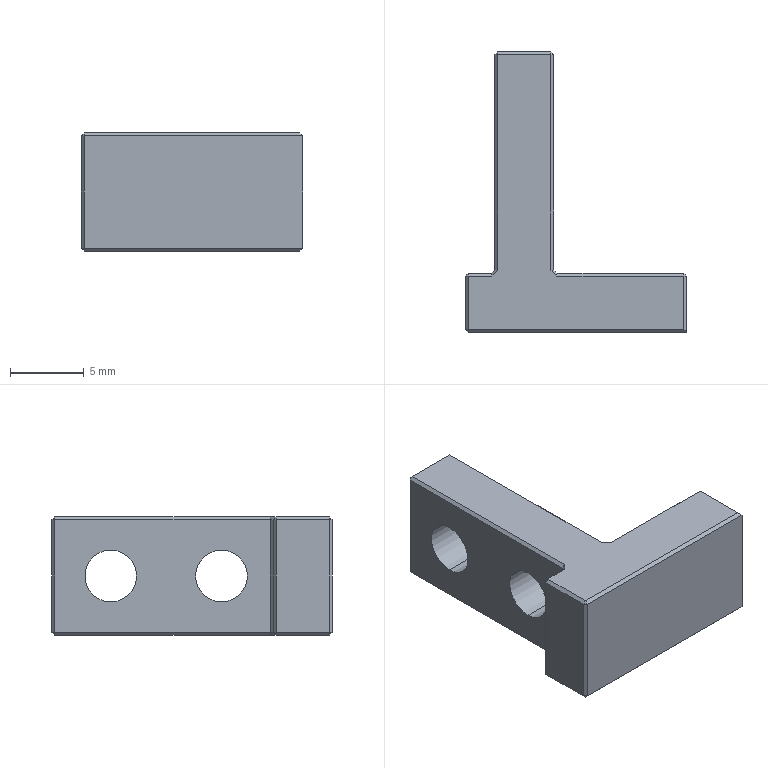Part | SolidWorks | features Chamfer 1, Extrusion 1, ICE 1 | 1 solid | 51 faces | box 15 x 19 x 8 mm | volume 879.9 mm3 | plane 47 | cylinder 4 | commonest cylinder face diameters 3.5 x4
STEP:
#1=CARTESIAN_POINT('',(-8.794,11.,2.25));
#2=VERTEX_POINT('',#1);
#3=CARTESIAN_POINT('',(-8.794,11.,5.75));
#4=VERTEX_POINT('',#3);
#5=CARTESIAN_POINT('',(-8.794,11.,4.));
#6=DIRECTION('',(-1.,0.,0.));
#7=DIRECTION('',(0.,0.,-1.));
#8=AXIS2_PLACEMENT_3D('',#5,#6,#7);
#9=CIRCLE('',#8,1.75);
#10=EDGE_CURVE('',#2,#4,#9,.T.);
#11=ORIENTED_EDGE('',*,*,#10,.T.);
#12=CARTESIAN_POINT('',(-4.794,11.,5.75));
#13=VERTEX_POINT('',#12);
#14=CARTESIAN_POINT('',(-10.794,11.,5.75));
#15=DIRECTION('',(1.,0.,0.));
#16=VECTOR('',#15,1000.);
#17=LINE('',#14,#16);
#18=EDGE_CURVE('',#4,#13,#17,.T.);
#19=ORIENTED_EDGE('',*,*,#18,.T.);
#20=CARTESIAN_POINT('',(-4.794,11.,2.25));
#21=VERTEX_POINT('',#20);
#22=CARTESIAN_POINT('',(-4.794,11.,4.));
#23=DIRECTION('',(1.,0.,0.));
#24=DIRECTION('',(0.,-1.,0.));
#25=AXIS2_PLACEMENT_3D('',#22,#23,#24);
#26=CIRCLE('',#25,1.75);
#27=EDGE_CURVE('',#13,#21,#26,.T.);
#28=ORIENTED_EDGE('',*,*,#27,.T.);
#29=CARTESIAN_POINT('',(-10.794,11.,2.25));
#30=DIRECTION('',(1.,0.,0.));
#31=VECTOR('',#30,1000.);
#32=LINE('',#29,#31);
#33=EDGE_CURVE('',#2,#21,#32,.T.);
#34=ORIENTED_EDGE('',*,*,#33,.F.);
#35=EDGE_LOOP('',(#11,#19,#28,#34));
#36=FACE_OUTER_BOUND('',#35,.T.);
#37=CARTESIAN_POINT('',(-10.794,11.,4.));
#38=DIRECTION('',(1.,0.,0.));
#39=DIRECTION('',(0.,0.,-1.));
#40=AXIS2_PLACEMENT_3D('',#37,#38,#39);
#41=CYLINDRICAL_SURFACE('',#40,1.75);
#42=ADVANCED_FACE('',(#36),#41,.F.);
#43=CARTESIAN_POINT('',(-8.794,3.5,2.25));
#44=VERTEX_POINT('',#43);
#45=CARTESIAN_POINT('',(-8.794,3.5,5.75));
#46=VERTEX_POINT('',#45);
#47=CARTESIAN_POINT('',(-8.794,3.5,4.));
#48=DIRECTION('',(-1.,0.,0.));
#49=DIRECTION('',(0.,0.,-1.));
#50=AXIS2_PLACEMENT_3D('',#47,#48,#49);
#51=CIRCLE('',#50,1.75);
#52=EDGE_CURVE('',#44,#46,#51,.T.);
#53=ORIENTED_EDGE('',*,*,#52,.T.);
#54=CARTESIAN_POINT('',(-4.794,3.5,5.75));
#55=VERTEX_POINT('',#54);
#56=CARTESIAN_POINT('',(-10.794,3.5,5.75));
#57=DIRECTION('',(1.,0.,0.));
#58=VECTOR('',#57,1000.);
#59=LINE('',#56,#58);
#60=EDGE_CURVE('',#46,#55,#59,.T.);
#61=ORIENTED_EDGE('',*,*,#60,.T.);
#62=CARTESIAN_POINT('',(-4.794,3.5,2.25));
#63=VERTEX_POINT('',#62);
#64=CARTESIAN_POINT('',(-4.794,3.5,4.));
#65=DIRECTION('',(1.,0.,0.));
#66=DIRECTION('',(0.,-1.,0.));
#67=AXIS2_PLACEMENT_3D('',#64,#65,#66);
#68=CIRCLE('',#67,1.75);
#69=EDGE_CURVE('',#55,#63,#68,.T.);
#70=ORIENTED_EDGE('',*,*,#69,.T.);
#71=CARTESIAN_POINT('',(-10.794,3.5,2.25));
#72=DIRECTION('',(1.,0.,0.));
#73=VECTOR('',#72,1000.);
#74=LINE('',#71,#73);
#75=EDGE_CURVE('',#44,#63,#74,.T.);
#76=ORIENTED_EDGE('',*,*,#75,.F.);
#77=EDGE_LOOP('',(#53,#61,#70,#76));
#78=FACE_OUTER_BOUND('',#77,.T.);
#79=CARTESIAN_POINT('',(-10.794,3.5,4.));
#80=DIRECTION('',(1.,0.,0.));
#81=DIRECTION('',(0.,0.,-1.));
#82=AXIS2_PLACEMENT_3D('',#79,#80,#81);
#83=CYLINDRICAL_SURFACE('',#82,1.75);
#84=ADVANCED_FACE('',(#78),#83,.F.);
#85=CARTESIAN_POINT('',(-8.594,14.8,8.));
#86=VERTEX_POINT('',#85);
#87=CARTESIAN_POINT('',(-8.594,0.2,8.));
#88=VERTEX_POINT('',#87);
#89=CARTESIAN_POINT('',(-8.594,0.,8.));
#90=DIRECTION('',(0.,-1.,0.));
#91=VECTOR('',#90,1000.);
#92=LINE('',#89,#91);
#93=EDGE_CURVE('',#86,#88,#92,.T.);
#94=ORIENTED_EDGE('',*,*,#93,.T.);
#95=CARTESIAN_POINT('',(-8.994,-0.2,8.));
#96=VERTEX_POINT('',#95);
#97=CARTESIAN_POINT('',(-4.397,4.397,8.));
#98=DIRECTION('',(0.7071,0.7071,0.));
#99=VECTOR('',#98,1000.);
#100=LINE('',#97,#99);
#101=EDGE_CURVE('',#96,#88,#100,.T.);
#102=ORIENTED_EDGE('',*,*,#101,.F.);
#103=CARTESIAN_POINT('',(-10.594,-0.2,8.));
#104=VERTEX_POINT('',#103);
#105=CARTESIAN_POINT('',(-10.794,-0.2,8.));
#106=DIRECTION('',(-1.,0.,0.));
#107=VECTOR('',#106,1000.);
#108=LINE('',#105,#107);
#109=EDGE_CURVE('',#96,#104,#108,.T.);
#110=ORIENTED_EDGE('',*,*,#109,.T.);
#111=CARTESIAN_POINT('',(-10.594,-3.8,8.));
#112=VERTEX_POINT('',#111);
#113=CARTESIAN_POINT('',(-10.594,-4.,8.));
#114=DIRECTION('',(0.,-1.,0.));
#115=VECTOR('',#114,1000.);
#116=LINE('',#113,#115);
#117=EDGE_CURVE('',#104,#112,#116,.T.);
#118=ORIENTED_EDGE('',*,*,#117,.T.);
#119=CARTESIAN_POINT('',(4.006,-3.8,8.));
#120=VERTEX_POINT('',#119);
#121=CARTESIAN_POINT('',(4.206,-3.8,8.));
#122=DIRECTION('',(1.,0.,0.));
#123=VECTOR('',#122,1000.);
#124=LINE('',#121,#123);
#125=EDGE_CURVE('',#112,#120,#124,.T.);
#126=ORIENTED_EDGE('',*,*,#125,.T.);
#127=CARTESIAN_POINT('',(4.006,-0.2,8.));
#128=VERTEX_POINT('',#127);
#129=CARTESIAN_POINT('',(4.006,0.,8.));
#130=DIRECTION('',(0.,1.,0.));
#131=VECTOR('',#130,1000.);
#132=LINE('',#129,#131);
#133=EDGE_CURVE('',#120,#128,#132,.T.);
#134=ORIENTED_EDGE('',*,*,#133,.T.);
#135=CARTESIAN_POINT('',(-4.594,-0.2,8.));
#136=VERTEX_POINT('',#135);
#137=CARTESIAN_POINT('',(-4.794,-0.2,8.));
#138=DIRECTION('',(-1.,0.,0.));
#139=VECTOR('',#138,1000.);
#140=LINE('',#137,#139);
#141=EDGE_CURVE('',#128,#136,#140,.T.);
#142=ORIENTED_EDGE('',*,*,#141,.T.);
#143=CARTESIAN_POINT('',(-4.994,0.2,8.));
#144=VERTEX_POINT('',#143);
#145=CARTESIAN_POINT('',(-2.397,-2.397,8.));
#146=DIRECTION('',(0.7071,-0.7071,0.));
#147=VECTOR('',#146,1000.);
#148=LINE('',#145,#147);
#149=EDGE_CURVE('',#144,#136,#148,.T.);
#150=ORIENTED_EDGE('',*,*,#149,.F.);
#151=CARTESIAN_POINT('',(-4.994,14.8,8.));
#152=VERTEX_POINT('',#151);
#153=CARTESIAN_POINT('',(-4.994,15.,8.));
#154=DIRECTION('',(0.,1.,0.));
#155=VECTOR('',#154,1000.);
#156=LINE('',#153,#155);
#157=EDGE_CURVE('',#144,#152,#156,.T.);
#158=ORIENTED_EDGE('',*,*,#157,.T.);
#159=CARTESIAN_POINT('',(-8.794,14.8,8.));
#160=DIRECTION('',(-1.,0.,0.));
#161=VECTOR('',#160,1000.);
#162=LINE('',#159,#161);
#163=EDGE_CURVE('',#152,#86,#162,.T.);
#164=ORIENTED_EDGE('',*,*,#163,.T.);
#165=EDGE_LOOP('',(#94,#102,#110,#118,#126,#134,#142,#150,#158,#164));
#166=FACE_OUTER_BOUND('',#165,.T.);
#167=CARTESIAN_POINT('',(0.,0.,8.));
#168=DIRECTION('',(0.,0.,1.));
#169=DIRECTION('',(1.,0.,0.));
#170=AXIS2_PLACEMENT_3D('',#167,#168,#169);
#171=PLANE('',#170);
#172=ADVANCED_FACE('',(#166),#171,.T.);
#173=CARTESIAN_POINT('',(-8.594,0.2,0.));
#174=VERTEX_POINT('',#173);
#175=CARTESIAN_POINT('',(-8.994,-0.2,0.));
#176=VERTEX_POINT('',#175);
#177=CARTESIAN_POINT('',(-8.994,-0.2,0.));
#178=DIRECTION('',(-0.7071,-0.7071,0.));
#179=VECTOR('',#178,1000.);
#180=LINE('',#177,#179);
#181=EDGE_CURVE('',#174,#176,#180,.T.);
#182=ORIENTED_EDGE('',*,*,#181,.F.);
#183=CARTESIAN_POINT('',(-8.594,14.8,0.));
#184=VERTEX_POINT('',#183);
#185=CARTESIAN_POINT('',(-8.594,0.,0.));
#186=DIRECTION('',(0.,1.,0.));
#187=VECTOR('',#186,1000.);
#188=LINE('',#185,#187);
#189=EDGE_CURVE('',#174,#184,#188,.T.);
#190=ORIENTED_EDGE('',*,*,#189,.T.);
#191=CARTESIAN_POINT('',(-4.994,14.8,0.));
#192=VERTEX_POINT('',#191);
#193=CARTESIAN_POINT('',(0.,14.8,0.));
#194=DIRECTION('',(1.,0.,0.));
#195=VECTOR('',#194,1000.);
#196=LINE('',#193,#195);
#197=EDGE_CURVE('',#184,#192,#196,.T.);
#198=ORIENTED_EDGE('',*,*,#197,.T.);
#199=CARTESIAN_POINT('',(-4.994,0.2,0.));
#200=VERTEX_POINT('',#199);
#201=CARTESIAN_POINT('',(-4.994,0.,0.));
#202=DIRECTION('',(0.,-1.,0.));
#203=VECTOR('',#202,1000.);
#204=LINE('',#201,#203);
#205=EDGE_CURVE('',#192,#200,#204,.T.);
#206=ORIENTED_EDGE('',*,*,#205,.T.);
#207=CARTESIAN_POINT('',(-4.594,-0.2,0.));
#208=VERTEX_POINT('',#207);
#209=CARTESIAN_POINT('',(-4.994,0.2,0.));
#210=DIRECTION('',(-0.7071,0.7071,0.));
#211=VECTOR('',#210,1000.);
#212=LINE('',#209,#211);
#213=EDGE_CURVE('',#208,#200,#212,.T.);
#214=ORIENTED_EDGE('',*,*,#213,.F.);
#215=CARTESIAN_POINT('',(4.006,-0.2,0.));
#216=VERTEX_POINT('',#215);
#217=CARTESIAN_POINT('',(0.,-0.2,0.));
#218=DIRECTION('',(1.,0.,0.));
#219=VECTOR('',#218,1000.);
#220=LINE('',#217,#219);
#221=EDGE_CURVE('',#208,#216,#220,.T.);
#222=ORIENTED_EDGE('',*,*,#221,.T.);
#223=CARTESIAN_POINT('',(4.006,-3.8,0.));
#224=VERTEX_POINT('',#223);
#225=CARTESIAN_POINT('',(4.006,0.,0.));
#226=DIRECTION('',(0.,-1.,0.));
#227=VECTOR('',#226,1000.);
#228=LINE('',#225,#227);
#229=EDGE_CURVE('',#216,#224,#228,.T.);
#230=ORIENTED_EDGE('',*,*,#229,.T.);
#231=CARTESIAN_POINT('',(-10.594,-3.8,0.));
#232=VERTEX_POINT('',#231);
#233=CARTESIAN_POINT('',(0.,-3.8,0.));
#234=DIRECTION('',(-1.,0.,0.));
#235=VECTOR('',#234,1000.);
#236=LINE('',#233,#235);
#237=EDGE_CURVE('',#224,#232,#236,.T.);
#238=ORIENTED_EDGE('',*,*,#237,.T.);
#239=CARTESIAN_POINT('',(-10.594,-0.2,0.));
#240=VERTEX_POINT('',#239);
#241=CARTESIAN_POINT('',(-10.594,0.,0.));
#242=DIRECTION('',(0.,1.,0.));
#243=VECTOR('',#242,1000.);
#244=LINE('',#241,#243);
#245=EDGE_CURVE('',#232,#240,#244,.T.);
#246=ORIENTED_EDGE('',*,*,#245,.T.);
#247=CARTESIAN_POINT('',(0.,-0.2,0.));
#248=DIRECTION('',(1.,0.,0.));
#249=VECTOR('',#248,1000.);
#250=LINE('',#247,#249);
#251=EDGE_CURVE('',#240,#176,#250,.T.);
#252=ORIENTED_EDGE('',*,*,#251,.T.);
#253=EDGE_LOOP('',(#182,#190,#198,#206,#214,#222,#230,#238,#246,#252));
#254=FACE_OUTER_BOUND('',#253,.T.);
#255=CARTESIAN_POINT('',(0.,0.,0.));
#256=DIRECTION('',(0.,0.,1.));
#257=DIRECTION('',(1.,0.,0.));
#258=AXIS2_PLACEMENT_3D('',#255,#256,#257);
#259=PLANE('',#258);
#260=ADVANCED_FACE('',(#254),#259,.F.);
#261=CARTESIAN_POINT('',(-10.794,-0.2,0.2));
#262=VERTEX_POINT('',#261);
#263=CARTESIAN_POINT('',(-10.794,-3.8,0.2));
#264=VERTEX_POINT('',#263);
#265=CARTESIAN_POINT('',(-10.794,0.,0.2));
#266=DIRECTION('',(0.,-1.,0.));
#267=VECTOR('',#266,1000.);
#268=LINE('',#265,#267);
#269=EDGE_CURVE('',#262,#264,#268,.T.);
#270=ORIENTED_EDGE('',*,*,#269,.T.);
#271=CARTESIAN_POINT('',(-10.794,-3.8,7.8));
#272=VERTEX_POINT('',#271);
#273=CARTESIAN_POINT('',(-10.794,-3.8,8.));
#274=DIRECTION('',(0.,0.,1.));
#275=VECTOR('',#274,1000.);
#276=LINE('',#273,#275);
#277=EDGE_CURVE('',#264,#272,#276,.T.);
#278=ORIENTED_EDGE('',*,*,#277,.T.);
#279=CARTESIAN_POINT('',(-10.794,-0.2,7.8));
#280=VERTEX_POINT('',#279);
#281=CARTESIAN_POINT('',(-10.794,0.,7.8));
#282=DIRECTION('',(0.,1.,0.));
#283=VECTOR('',#282,1000.);
#284=LINE('',#281,#283);
#285=EDGE_CURVE('',#272,#280,#284,.T.);
#286=ORIENTED_EDGE('',*,*,#285,.T.);
#287=CARTESIAN_POINT('',(-10.794,-0.2,8.));
#288=DIRECTION('',(0.,0.,-1.));
#289=VECTOR('',#288,1000.);
#290=LINE('',#287,#289);
#291=EDGE_CURVE('',#280,#262,#290,.T.);
#292=ORIENTED_EDGE('',*,*,#291,.T.);
#293=EDGE_LOOP('',(#270,#278,#286,#292));
#294=FACE_OUTER_BOUND('',#293,.T.);
#295=CARTESIAN_POINT('',(-10.794,0.,8.));
#296=DIRECTION('',(1.,0.,0.));
#297=DIRECTION('',(0.,0.,-1.));
#298=AXIS2_PLACEMENT_3D('',#295,#296,#297);
#299=PLANE('',#298);
#300=ADVANCED_FACE('',(#294),#299,.F.);
#301=CARTESIAN_POINT('',(-10.594,-4.,7.8));
#302=VERTEX_POINT('',#301);
#303=CARTESIAN_POINT('',(-10.594,-4.,0.2));
#304=VERTEX_POINT('',#303);
#305=CARTESIAN_POINT('',(-10.594,-4.,8.));
#306=DIRECTION('',(0.,0.,-1.));
#307=VECTOR('',#306,1000.);
#308=LINE('',#305,#307);
#309=EDGE_CURVE('',#302,#304,#308,.T.);
#310=ORIENTED_EDGE('',*,*,#309,.T.);
#311=CARTESIAN_POINT('',(4.206,-4.,0.2));
#312=VERTEX_POINT('',#311);
#313=CARTESIAN_POINT('',(-10.794,-4.,0.2));
#314=DIRECTION('',(1.,0.,0.));
#315=VECTOR('',#314,1000.);
#316=LINE('',#313,#315);
#317=EDGE_CURVE('',#304,#312,#316,.T.);
#318=ORIENTED_EDGE('',*,*,#317,.T.);
#319=CARTESIAN_POINT('',(4.206,-4.,7.8));
#320=VERTEX_POINT('',#319);
#321=CARTESIAN_POINT('',(4.206,-4.,8.));
#322=DIRECTION('',(0.,0.,-1.));
#323=VECTOR('',#322,1000.);
#324=LINE('',#321,#323);
#325=EDGE_CURVE('',#320,#312,#324,.T.);
#326=ORIENTED_EDGE('',*,*,#325,.F.);
#327=CARTESIAN_POINT('',(-10.794,-4.,7.8));
#328=DIRECTION('',(-1.,0.,0.));
#329=VECTOR('',#328,1000.);
#330=LINE('',#327,#329);
#331=EDGE_CURVE('',#320,#302,#330,.T.);
#332=ORIENTED_EDGE('',*,*,#331,.T.);
#333=EDGE_LOOP('',(#310,#318,#326,#332));
#334=FACE_OUTER_BOUND('',#333,.T.);
#335=CARTESIAN_POINT('',(-10.794,-4.,8.));
#336=DIRECTION('',(0.,1.,0.));
#337=DIRECTION('',(0.,0.,1.));
#338=AXIS2_PLACEMENT_3D('',#335,#336,#337);
#339=PLANE('',#338);
#340=ADVANCED_FACE('',(#334),#339,.F.);
#341=ORIENTED_EDGE('',*,*,#325,.T.);
#342=CARTESIAN_POINT('',(4.206,-0.2,0.2));
#343=VERTEX_POINT('',#342);
#344=CARTESIAN_POINT('',(4.206,-4.,0.2));
#345=DIRECTION('',(0.,1.,0.));
#346=VECTOR('',#345,1000.);
#347=LINE('',#344,#346);
#348=EDGE_CURVE('',#312,#343,#347,.T.);
#349=ORIENTED_EDGE('',*,*,#348,.T.);
#350=CARTESIAN_POINT('',(4.206,-0.2,7.8));
#351=VERTEX_POINT('',#350);
#352=CARTESIAN_POINT('',(4.206,-0.2,8.));
#353=DIRECTION('',(0.,0.,1.));
#354=VECTOR('',#353,1000.);
#355=LINE('',#352,#354);
#356=EDGE_CURVE('',#343,#351,#355,.T.);
#357=ORIENTED_EDGE('',*,*,#356,.T.);
#358=CARTESIAN_POINT('',(4.206,-4.,7.8));
#359=DIRECTION('',(0.,-1.,0.));
#360=VECTOR('',#359,1000.);
#361=LINE('',#358,#360);
#362=EDGE_CURVE('',#351,#320,#361,.T.);
#363=ORIENTED_EDGE('',*,*,#362,.T.);
#364=EDGE_LOOP('',(#341,#349,#357,#363));
#365=FACE_OUTER_BOUND('',#364,.T.);
#366=CARTESIAN_POINT('',(4.206,-4.,8.));
#367=DIRECTION('',(-1.,0.,0.));
#368=DIRECTION('',(0.,-1.,0.));
#369=AXIS2_PLACEMENT_3D('',#366,#367,#368);
#370=PLANE('',#369);
#371=ADVANCED_FACE('',(#365),#370,.F.);
#372=CARTESIAN_POINT('',(-4.594,0.,7.8));
#373=VERTEX_POINT('',#372);
#374=CARTESIAN_POINT('',(4.006,0.,7.8));
#375=VERTEX_POINT('',#374);
#376=CARTESIAN_POINT('',(4.206,0.,7.8));
#377=DIRECTION('',(1.,0.,0.));
#378=VECTOR('',#377,1000.);
#379=LINE('',#376,#378);
#380=EDGE_CURVE('',#373,#375,#379,.T.);
#381=ORIENTED_EDGE('',*,*,#380,.T.);
#382=CARTESIAN_POINT('',(4.006,0.,0.2));
#383=VERTEX_POINT('',#382);
#384=CARTESIAN_POINT('',(4.006,0.,8.));
#385=DIRECTION('',(0.,0.,-1.));
#386=VECTOR('',#385,1000.);
#387=LINE('',#384,#386);
#388=EDGE_CURVE('',#375,#383,#387,.T.);
#389=ORIENTED_EDGE('',*,*,#388,.T.);
#390=CARTESIAN_POINT('',(-4.594,0.,0.2));
#391=VERTEX_POINT('',#390);
#392=CARTESIAN_POINT('',(-4.794,0.,0.2));
#393=DIRECTION('',(-1.,0.,0.));
#394=VECTOR('',#393,1000.);
#395=LINE('',#392,#394);
#396=EDGE_CURVE('',#383,#391,#395,.T.);
#397=ORIENTED_EDGE('',*,*,#396,.T.);
#398=CARTESIAN_POINT('',(-4.594,0.,8.));
#399=DIRECTION('',(0.,0.,1.));
#400=VECTOR('',#399,1000.);
#401=LINE('',#398,#400);
#402=EDGE_CURVE('',#391,#373,#401,.T.);
#403=ORIENTED_EDGE('',*,*,#402,.T.);
#404=EDGE_LOOP('',(#381,#389,#397,#403));
#405=FACE_OUTER_BOUND('',#404,.T.);
#406=CARTESIAN_POINT('',(-4.794,0.,8.));
#407=DIRECTION('',(0.,-1.,0.));
#408=DIRECTION('',(0.,0.,-1.));
#409=AXIS2_PLACEMENT_3D('',#406,#407,#408);
#410=PLANE('',#409);
#411=ADVANCED_FACE('',(#405),#410,.F.);
#412=CARTESIAN_POINT('',(-4.794,11.,4.));
#413=DIRECTION('',(1.,0.,0.));
#414=DIRECTION('',(0.,-1.,0.));
#415=AXIS2_PLACEMENT_3D('',#412,#413,#414);
#416=CIRCLE('',#415,1.75);
#417=EDGE_CURVE('',#21,#13,#416,.T.);
#418=ORIENTED_EDGE('',*,*,#417,.F.);
#419=ORIENTED_EDGE('',*,*,#27,.F.);
#420=EDGE_LOOP('',(#418,#419));
#421=FACE_BOUND('',#420,.T.);
#422=CARTESIAN_POINT('',(-4.794,3.5,4.));
#423=DIRECTION('',(1.,0.,0.));
#424=DIRECTION('',(0.,-1.,0.));
#425=AXIS2_PLACEMENT_3D('',#422,#423,#424);
#426=CIRCLE('',#425,1.75);
#427=EDGE_CURVE('',#63,#55,#426,.T.);
#428=ORIENTED_EDGE('',*,*,#427,.F.);
#429=ORIENTED_EDGE('',*,*,#69,.F.);
#430=EDGE_LOOP('',(#428,#429));
#431=FACE_BOUND('',#430,.T.);
#432=CARTESIAN_POINT('',(-4.794,0.2,0.2));
#433=VERTEX_POINT('',#432);
#434=CARTESIAN_POINT('',(-4.794,14.8,0.2));
#435=VERTEX_POINT('',#434);
#436=CARTESIAN_POINT('',(-4.794,15.,0.2));
#437=DIRECTION('',(0.,1.,0.));
#438=VECTOR('',#437,1000.);
#439=LINE('',#436,#438);
#440=EDGE_CURVE('',#433,#435,#439,.T.);
#441=ORIENTED_EDGE('',*,*,#440,.T.);
#442=CARTESIAN_POINT('',(-4.794,14.8,7.8));
#443=VERTEX_POINT('',#442);
#444=CARTESIAN_POINT('',(-4.794,14.8,8.));
#445=DIRECTION('',(0.,0.,1.));
#446=VECTOR('',#445,1000.);
#447=LINE('',#444,#446);
#448=EDGE_CURVE('',#435,#443,#447,.T.);
#449=ORIENTED_EDGE('',*,*,#448,.T.);
#450=CARTESIAN_POINT('',(-4.794,0.2,7.8));
#451=VERTEX_POINT('',#450);
#452=CARTESIAN_POINT('',(-4.794,0.,7.8));
#453=DIRECTION('',(0.,-1.,0.));
#454=VECTOR('',#453,1000.);
#455=LINE('',#452,#454);
#456=EDGE_CURVE('',#443,#451,#455,.T.);
#457=ORIENTED_EDGE('',*,*,#456,.T.);
#458=CARTESIAN_POINT('',(-4.794,0.2,0.));
#459=DIRECTION('',(0.,0.,-1.));
#460=VECTOR('',#459,1000.);
#461=LINE('',#458,#460);
#462=EDGE_CURVE('',#451,#433,#461,.T.);
#463=ORIENTED_EDGE('',*,*,#462,.T.);
#464=EDGE_LOOP('',(#441,#449,#457,#463));
#465=FACE_OUTER_BOUND('',#464,.T.);
#466=CARTESIAN_POINT('',(-4.794,15.,8.));
#467=DIRECTION('',(-1.,0.,0.));
#468=DIRECTION('',(0.,-1.,0.));
#469=AXIS2_PLACEMENT_3D('',#466,#467,#468);
#470=PLANE('',#469);
#471=ADVANCED_FACE('',(#421,#431,#465),#470,.F.);
#472=CARTESIAN_POINT('',(-4.994,15.,7.8));
#473=VERTEX_POINT('',#472);
#474=CARTESIAN_POINT('',(-4.994,15.,0.2));
#475=VERTEX_POINT('',#474);
#476=CARTESIAN_POINT('',(-4.994,15.,8.));
#477=DIRECTION('',(0.,0.,-1.));
#478=VECTOR('',#477,1000.);
#479=LINE('',#476,#478);
#480=EDGE_CURVE('',#473,#475,#479,.T.);
#481=ORIENTED_EDGE('',*,*,#480,.T.);
#482=CARTESIAN_POINT('',(-8.594,15.,0.2));
#483=VERTEX_POINT('',#482);
#484=CARTESIAN_POINT('',(-8.794,15.,0.2));
#485=DIRECTION('',(-1.,0.,0.));
#486=VECTOR('',#485,1000.);
#487=LINE('',#484,#486);
#488=EDGE_CURVE('',#475,#483,#487,.T.);
#489=ORIENTED_EDGE('',*,*,#488,.T.);
#490=CARTESIAN_POINT('',(-8.594,15.,7.8));
#491=VERTEX_POINT('',#490);
#492=CARTESIAN_POINT('',(-8.594,15.,8.));
#493=DIRECTION('',(0.,0.,1.));
#494=VECTOR('',#493,1000.);
#495=LINE('',#492,#494);
#496=EDGE_CURVE('',#483,#491,#495,.T.);
#497=ORIENTED_EDGE('',*,*,#496,.T.);
#498=CARTESIAN_POINT('',(-4.794,15.,7.8));
#499=DIRECTION('',(1.,0.,0.));
#500=VECTOR('',#499,1000.);
#501=LINE('',#498,#500);
#502=EDGE_CURVE('',#491,#473,#501,.T.);
#503=ORIENTED_EDGE('',*,*,#502,.T.);
#504=EDGE_LOOP('',(#481,#489,#497,#503));
#505=FACE_OUTER_BOUND('',#504,.T.);
#506=CARTESIAN_POINT('',(-8.794,15.,8.));
#507=DIRECTION('',(0.,-1.,0.));
#508=DIRECTION('',(0.,0.,-1.));
#509=AXIS2_PLACEMENT_3D('',#506,#507,#508);
#510=PLANE('',#509);
#511=ADVANCED_FACE('',(#505),#510,.F.);
#512=ORIENTED_EDGE('',*,*,#10,.F.);
#513=CARTESIAN_POINT('',(-8.794,11.,4.));
#514=DIRECTION('',(-1.,0.,0.));
#515=DIRECTION('',(0.,0.,-1.));
#516=AXIS2_PLACEMENT_3D('',#513,#514,#515);
#517=CIRCLE('',#516,1.75);
#518=EDGE_CURVE('',#4,#2,#517,.T.);
#519=ORIENTED_EDGE('',*,*,#518,.F.);
#520=EDGE_LOOP('',(#512,#519));
#521=FACE_BOUND('',#520,.T.);
#522=ORIENTED_EDGE('',*,*,#52,.F.);
#523=CARTESIAN_POINT('',(-8.794,3.5,4.));
#524=DIRECTION('',(-1.,0.,0.));
#525=DIRECTION('',(0.,0.,-1.));
#526=AXIS2_PLACEMENT_3D('',#523,#524,#525);
#527=CIRCLE('',#526,1.75);
#528=EDGE_CURVE('',#46,#44,#527,.T.);
#529=ORIENTED_EDGE('',*,*,#528,.F.);
#530=EDGE_LOOP('',(#522,#529));
#531=FACE_BOUND('',#530,.T.);
#532=CARTESIAN_POINT('',(-8.794,0.2,7.8));
#533=VERTEX_POINT('',#532);
#534=CARTESIAN_POINT('',(-8.794,14.8,7.8));
#535=VERTEX_POINT('',#534);
#536=CARTESIAN_POINT('',(-8.794,15.,7.8));
#537=DIRECTION('',(0.,1.,0.));
#538=VECTOR('',#537,1000.);
#539=LINE('',#536,#538);
#540=EDGE_CURVE('',#533,#535,#539,.T.);
#541=ORIENTED_EDGE('',*,*,#540,.T.);
#542=CARTESIAN_POINT('',(-8.794,14.8,0.2));
#543=VERTEX_POINT('',#542);
#544=CARTESIAN_POINT('',(-8.794,14.8,8.));
#545=DIRECTION('',(0.,0.,-1.));
#546=VECTOR('',#545,1000.);
#547=LINE('',#544,#546);
#548=EDGE_CURVE('',#535,#543,#547,.T.);
#549=ORIENTED_EDGE('',*,*,#548,.T.);
#550=CARTESIAN_POINT('',(-8.794,0.2,0.2));
#551=VERTEX_POINT('',#550);
#552=CARTESIAN_POINT('',(-8.794,0.,0.2));
#553=DIRECTION('',(0.,-1.,0.));
#554=VECTOR('',#553,1000.);
#555=LINE('',#552,#554);
#556=EDGE_CURVE('',#543,#551,#555,.T.);
#557=ORIENTED_EDGE('',*,*,#556,.T.);
#558=CARTESIAN_POINT('',(-8.794,0.2,8.));
#559=DIRECTION('',(0.,0.,1.));
#560=VECTOR('',#559,1000.);
#561=LINE('',#558,#560);
#562=EDGE_CURVE('',#551,#533,#561,.T.);
#563=ORIENTED_EDGE('',*,*,#562,.T.);
#564=EDGE_LOOP('',(#541,#549,#557,#563));
#565=FACE_OUTER_BOUND('',#564,.T.);
#566=CARTESIAN_POINT('',(-8.794,0.,8.));
#567=DIRECTION('',(1.,0.,0.));
#568=DIRECTION('',(0.,0.,-1.));
#569=AXIS2_PLACEMENT_3D('',#566,#567,#568);
#570=PLANE('',#569);
#571=ADVANCED_FACE('',(#521,#531,#565),#570,.F.);
#572=CARTESIAN_POINT('',(-10.594,0.,7.8));
#573=VERTEX_POINT('',#572);
#574=CARTESIAN_POINT('',(-8.994,0.,7.8));
#575=VERTEX_POINT('',#574);
#576=CARTESIAN_POINT('',(-8.794,0.,7.8));
#577=DIRECTION('',(1.,0.,0.));
#578=VECTOR('',#577,1000.);
#579=LINE('',#576,#578);
#580=EDGE_CURVE('',#573,#575,#579,.T.);
#581=ORIENTED_EDGE('',*,*,#580,.T.);
#582=CARTESIAN_POINT('',(-8.994,0.,0.2));
#583=VERTEX_POINT('',#582);
#584=CARTESIAN_POINT('',(-8.994,0.,0.));
#585=DIRECTION('',(0.,0.,-1.));
#586=VECTOR('',#585,1000.);
#587=LINE('',#584,#586);
#588=EDGE_CURVE('',#575,#583,#587,.T.);
#589=ORIENTED_EDGE('',*,*,#588,.T.);
#590=CARTESIAN_POINT('',(-10.594,0.,0.2));
#591=VERTEX_POINT('',#590);
#592=CARTESIAN_POINT('',(-10.794,0.,0.2));
#593=DIRECTION('',(-1.,0.,0.));
#594=VECTOR('',#593,1000.);
#595=LINE('',#592,#594);
#596=EDGE_CURVE('',#583,#591,#595,.T.);
#597=ORIENTED_EDGE('',*,*,#596,.T.);
#598=CARTESIAN_POINT('',(-10.594,0.,8.));
#599=DIRECTION('',(0.,0.,1.));
#600=VECTOR('',#599,1000.);
#601=LINE('',#598,#600);
#602=EDGE_CURVE('',#591,#573,#601,.T.);
#603=ORIENTED_EDGE('',*,*,#602,.T.);
#604=EDGE_LOOP('',(#581,#589,#597,#603));
#605=FACE_OUTER_BOUND('',#604,.T.);
#606=CARTESIAN_POINT('',(-10.794,0.,8.));
#607=DIRECTION('',(0.,-1.,0.));
#608=DIRECTION('',(0.,0.,-1.));
#609=AXIS2_PLACEMENT_3D('',#606,#607,#608);
#610=PLANE('',#609);
#611=ADVANCED_FACE('',(#605),#610,.F.);
#612=CARTESIAN_POINT('',(-10.794,-3.8,7.8));
#613=DIRECTION('',(0.7071,-0.7071,0.));
#614=VECTOR('',#613,1000.);
#615=LINE('',#612,#614);
#616=EDGE_CURVE('',#272,#302,#615,.T.);
#617=ORIENTED_EDGE('',*,*,#616,.F.);
#618=ORIENTED_EDGE('',*,*,#277,.F.);
#619=CARTESIAN_POINT('',(-10.594,-4.,0.2));
#620=DIRECTION('',(-0.7071,0.7071,0.));
#621=VECTOR('',#620,1000.);
#622=LINE('',#619,#621);
#623=EDGE_CURVE('',#304,#264,#622,.T.);
#624=ORIENTED_EDGE('',*,*,#623,.F.);
#625=ORIENTED_EDGE('',*,*,#309,.F.);
#626=EDGE_LOOP('',(#617,#618,#624,#625));
#627=FACE_OUTER_BOUND('',#626,.T.);
#628=CARTESIAN_POINT('',(-10.594,-4.,8.));
#629=DIRECTION('',(0.7071,0.7071,0.));
#630=DIRECTION('',(0.,0.,-1.));
#631=AXIS2_PLACEMENT_3D('',#628,#629,#630);
#632=PLANE('',#631);
#633=ADVANCED_FACE('',(#627),#632,.F.);
#634=CARTESIAN_POINT('',(-10.594,-3.9,7.9));
#635=DIRECTION('',(0.,-0.7071,-0.7071));
#636=VECTOR('',#635,1000.);
#637=LINE('',#634,#636);
#638=EDGE_CURVE('',#112,#302,#637,.T.);
#639=ORIENTED_EDGE('',*,*,#638,.F.);
#640=CARTESIAN_POINT('',(-10.794,-3.8,7.8));
#641=DIRECTION('',(0.7071,0.,0.7071));
#642=VECTOR('',#641,1000.);
#643=LINE('',#640,#642);
#644=EDGE_CURVE('',#272,#112,#643,.T.);
#645=ORIENTED_EDGE('',*,*,#644,.F.);
#646=ORIENTED_EDGE('',*,*,#616,.T.);
#647=EDGE_LOOP('',(#639,#645,#646));
#648=FACE_OUTER_BOUND('',#647,.T.);
#649=CARTESIAN_POINT('',(-10.794,-3.8,7.8));
#650=DIRECTION('',(-0.5774,-0.5774,0.5774));
#651=DIRECTION('',(0.7071,0.,0.7071));
#652=AXIS2_PLACEMENT_3D('',#649,#650,#651);
#653=PLANE('',#652);
#654=ADVANCED_FACE('',(#648),#653,.T.);
#655=ORIENTED_EDGE('',*,*,#644,.T.);
#656=ORIENTED_EDGE('',*,*,#117,.F.);
#657=CARTESIAN_POINT('',(-10.694,-0.2,7.9));
#658=DIRECTION('',(0.7071,0.,0.7071));
#659=VECTOR('',#658,1000.);
#660=LINE('',#657,#659);
#661=EDGE_CURVE('',#280,#104,#660,.T.);
#662=ORIENTED_EDGE('',*,*,#661,.F.);
#663=ORIENTED_EDGE('',*,*,#285,.F.);
#664=EDGE_LOOP('',(#655,#656,#662,#663));
#665=FACE_OUTER_BOUND('',#664,.T.);
#666=CARTESIAN_POINT('',(-10.594,0.,8.));
#667=DIRECTION('',(-0.7071,0.,0.7071));
#668=DIRECTION('',(0.,1.,0.));
#669=AXIS2_PLACEMENT_3D('',#666,#667,#668);
#670=PLANE('',#669);
#671=ADVANCED_FACE('',(#665),#670,.T.);
#672=CARTESIAN_POINT('',(-10.694,-0.1,0.2));
#673=DIRECTION('',(0.7071,0.7071,0.));
#674=VECTOR('',#673,1000.);
#675=LINE('',#672,#674);
#676=EDGE_CURVE('',#262,#591,#675,.T.);
#677=ORIENTED_EDGE('',*,*,#676,.F.);
#678=ORIENTED_EDGE('',*,*,#291,.F.);
#679=CARTESIAN_POINT('',(-10.594,0.,7.8));
#680=DIRECTION('',(-0.7071,-0.7071,0.));
#681=VECTOR('',#680,1000.);
#682=LINE('',#679,#681);
#683=EDGE_CURVE('',#573,#280,#682,.T.);
#684=ORIENTED_EDGE('',*,*,#683,.F.);
#685=ORIENTED_EDGE('',*,*,#602,.F.);
#686=EDGE_LOOP('',(#677,#678,#684,#685));
#687=FACE_OUTER_BOUND('',#686,.T.);
#688=CARTESIAN_POINT('',(-10.794,-0.2,8.));
#689=DIRECTION('',(0.7071,-0.7071,0.));
#690=DIRECTION('',(0.,0.,-1.));
#691=AXIS2_PLACEMENT_3D('',#688,#689,#690);
#692=PLANE('',#691);
#693=ADVANCED_FACE('',(#687),#692,.F.);
#694=CARTESIAN_POINT('',(-10.694,-3.8,0.1));
#695=DIRECTION('',(0.7071,0.,-0.7071));
#696=VECTOR('',#695,1000.);
#697=LINE('',#694,#696);
#698=EDGE_CURVE('',#264,#232,#697,.T.);
#699=ORIENTED_EDGE('',*,*,#698,.F.);
#700=ORIENTED_EDGE('',*,*,#269,.F.);
#701=CARTESIAN_POINT('',(-10.594,-0.2,0.));
#702=DIRECTION('',(-0.7071,0.,0.7071));
#703=VECTOR('',#702,1000.);
#704=LINE('',#701,#703);
#705=EDGE_CURVE('',#240,#262,#704,.T.);
#706=ORIENTED_EDGE('',*,*,#705,.F.);
#707=ORIENTED_EDGE('',*,*,#245,.F.);
#708=EDGE_LOOP('',(#699,#700,#706,#707));
#709=FACE_OUTER_BOUND('',#708,.T.);
#710=CARTESIAN_POINT('',(-10.794,0.,0.2));
#711=DIRECTION('',(0.7071,0.,0.7071));
#712=DIRECTION('',(0.,-1.,0.));
#713=AXIS2_PLACEMENT_3D('',#710,#711,#712);
#714=PLANE('',#713);
#715=ADVANCED_FACE('',(#709),#714,.F.);
#716=ORIENTED_EDGE('',*,*,#623,.T.);
#717=ORIENTED_EDGE('',*,*,#698,.T.);
#718=CARTESIAN_POINT('',(-10.594,-4.,0.2));
#719=DIRECTION('',(0.,0.7071,-0.7071));
#720=VECTOR('',#719,1000.);
#721=LINE('',#718,#720);
#722=EDGE_CURVE('',#304,#232,#721,.T.);
#723=ORIENTED_EDGE('',*,*,#722,.F.);
#724=EDGE_LOOP('',(#716,#717,#723));
#725=FACE_OUTER_BOUND('',#724,.T.);
#726=CARTESIAN_POINT('',(-10.594,-4.,0.2));
#727=DIRECTION('',(-0.5774,-0.5774,-0.5774));
#728=DIRECTION('',(-0.7071,0.,0.7071));
#729=AXIS2_PLACEMENT_3D('',#726,#727,#728);
#730=PLANE('',#729);
#731=ADVANCED_FACE('',(#725),#730,.T.);
#732=ORIENTED_EDGE('',*,*,#638,.T.);
#733=ORIENTED_EDGE('',*,*,#331,.F.);
#734=CARTESIAN_POINT('',(2.671,-2.465,9.335));
#735=DIRECTION('',(0.5774,-0.5774,-0.5774));
#736=VECTOR('',#735,1000.);
#737=LINE('',#734,#736);
#738=EDGE_CURVE('',#120,#320,#737,.T.);
#739=ORIENTED_EDGE('',*,*,#738,.F.);
#740=ORIENTED_EDGE('',*,*,#125,.F.);
#741=EDGE_LOOP('',(#732,#733,#739,#740));
#742=FACE_OUTER_BOUND('',#741,.T.);
#743=CARTESIAN_POINT('',(0.,-3.8,8.));
#744=DIRECTION('',(0.,-0.7071,0.7071));
#745=DIRECTION('',(-1.,0.,0.));
#746=AXIS2_PLACEMENT_3D('',#743,#744,#745);
#747=PLANE('',#746);
#748=ADVANCED_FACE('',(#742),#747,.T.);
#749=ORIENTED_EDGE('',*,*,#683,.T.);
#750=ORIENTED_EDGE('',*,*,#661,.T.);
#751=CARTESIAN_POINT('',(-10.594,0.,7.8));
#752=DIRECTION('',(0.,-0.7071,0.7071));
#753=VECTOR('',#752,1000.);
#754=LINE('',#751,#753);
#755=EDGE_CURVE('',#573,#104,#754,.T.);
#756=ORIENTED_EDGE('',*,*,#755,.F.);
#757=EDGE_LOOP('',(#749,#750,#756));
#758=FACE_OUTER_BOUND('',#757,.T.);
#759=CARTESIAN_POINT('',(-10.594,0.,7.8));
#760=DIRECTION('',(-0.5774,0.5774,0.5774));
#761=DIRECTION('',(0.7071,0.,0.7071));
#762=AXIS2_PLACEMENT_3D('',#759,#760,#761);
#763=PLANE('',#762);
#764=ADVANCED_FACE('',(#758),#763,.T.);
#765=ORIENTED_EDGE('',*,*,#705,.T.);
#766=ORIENTED_EDGE('',*,*,#676,.T.);
#767=CARTESIAN_POINT('',(-10.594,-0.2,0.));
#768=DIRECTION('',(0.,0.7071,0.7071));
#769=VECTOR('',#768,1000.);
#770=LINE('',#767,#769);
#771=EDGE_CURVE('',#240,#591,#770,.T.);
#772=ORIENTED_EDGE('',*,*,#771,.F.);
#773=EDGE_LOOP('',(#765,#766,#772));
#774=FACE_OUTER_BOUND('',#773,.T.);
#775=CARTESIAN_POINT('',(-10.594,-0.2,0.));
#776=DIRECTION('',(-0.5774,0.5774,-0.5774));
#777=DIRECTION('',(-0.7071,0.,0.7071));
#778=AXIS2_PLACEMENT_3D('',#775,#776,#777);
#779=PLANE('',#778);
#780=ADVANCED_FACE('',(#774),#779,.T.);
#781=ORIENTED_EDGE('',*,*,#722,.T.);
#782=ORIENTED_EDGE('',*,*,#237,.F.);
#783=CARTESIAN_POINT('',(4.206,-4.,0.2));
#784=DIRECTION('',(-0.5774,0.5774,-0.5774));
#785=VECTOR('',#784,1000.);
#786=LINE('',#783,#785);
#787=EDGE_CURVE('',#312,#224,#786,.T.);
#788=ORIENTED_EDGE('',*,*,#787,.F.);
#789=ORIENTED_EDGE('',*,*,#317,.F.);
#790=EDGE_LOOP('',(#781,#782,#788,#789));
#791=FACE_OUTER_BOUND('',#790,.T.);
#792=CARTESIAN_POINT('',(-10.794,-4.,0.2));
#793=DIRECTION('',(0.,0.7071,0.7071));
#794=DIRECTION('',(1.,0.,0.));
#795=AXIS2_PLACEMENT_3D('',#792,#793,#794);
#796=PLANE('',#795);
#797=ADVANCED_FACE('',(#791),#796,.F.);
#798=ORIENTED_EDGE('',*,*,#738,.T.);
#799=ORIENTED_EDGE('',*,*,#362,.F.);
#800=CARTESIAN_POINT('',(4.206,-0.2,7.8));
#801=DIRECTION('',(0.7071,0.,-0.7071));
#802=VECTOR('',#801,1000.);
#803=LINE('',#800,#802);
#804=EDGE_CURVE('',#128,#351,#803,.T.);
#805=ORIENTED_EDGE('',*,*,#804,.F.);
#806=ORIENTED_EDGE('',*,*,#133,.F.);
#807=EDGE_LOOP('',(#798,#799,#805,#806));
#808=FACE_OUTER_BOUND('',#807,.T.);
#809=CARTESIAN_POINT('',(4.006,0.,8.));
#810=DIRECTION('',(0.7071,0.,0.7071));
#811=DIRECTION('',(0.,-1.,0.));
#812=AXIS2_PLACEMENT_3D('',#809,#810,#811);
#813=PLANE('',#812);
#814=ADVANCED_FACE('',(#808),#813,.T.);
#815=ORIENTED_EDGE('',*,*,#755,.T.);
#816=ORIENTED_EDGE('',*,*,#109,.F.);
#817=CARTESIAN_POINT('',(-8.994,0.,7.8));
#818=DIRECTION('',(0.,-0.7071,0.7071));
#819=VECTOR('',#818,1000.);
#820=LINE('',#817,#819);
#821=EDGE_CURVE('',#575,#96,#820,.T.);
#822=ORIENTED_EDGE('',*,*,#821,.F.);
#823=ORIENTED_EDGE('',*,*,#580,.F.);
#824=EDGE_LOOP('',(#815,#816,#822,#823));
#825=FACE_OUTER_BOUND('',#824,.T.);
#826=CARTESIAN_POINT('',(0.,-0.2,8.));
#827=DIRECTION('',(0.,0.7071,0.7071));
#828=DIRECTION('',(1.,0.,0.));
#829=AXIS2_PLACEMENT_3D('',#826,#827,#828);
#830=PLANE('',#829);
#831=ADVANCED_FACE('',(#825),#830,.T.);
#832=CARTESIAN_POINT('',(-8.994,0.,0.2));
#833=DIRECTION('',(0.7071,0.7071,0.));
#834=VECTOR('',#833,1000.);
#835=LINE('',#832,#834);
#836=EDGE_CURVE('',#583,#551,#835,.T.);
#837=ORIENTED_EDGE('',*,*,#836,.F.);
#838=ORIENTED_EDGE('',*,*,#588,.F.);
#839=CARTESIAN_POINT('',(-8.994,0.,7.8));
#840=DIRECTION('',(-0.7071,-0.7071,0.));
#841=VECTOR('',#840,1000.);
#842=LINE('',#839,#841);
#843=EDGE_CURVE('',#533,#575,#842,.T.);
#844=ORIENTED_EDGE('',*,*,#843,.F.);
#845=ORIENTED_EDGE('',*,*,#562,.F.);
#846=EDGE_LOOP('',(#837,#838,#844,#845));
#847=FACE_OUTER_BOUND('',#846,.T.);
#848=CARTESIAN_POINT('',(-8.994,0.,8.));
#849=DIRECTION('',(-0.7071,0.7071,0.));
#850=DIRECTION('',(0.,0.,1.));
#851=AXIS2_PLACEMENT_3D('',#848,#849,#850);
#852=PLANE('',#851);
#853=ADVANCED_FACE('',(#847),#852,.T.);
#854=ORIENTED_EDGE('',*,*,#771,.T.);
#855=ORIENTED_EDGE('',*,*,#596,.F.);
#856=CARTESIAN_POINT('',(-8.994,-0.2,0.));
#857=DIRECTION('',(0.,0.7071,0.7071));
#858=VECTOR('',#857,1000.);
#859=LINE('',#856,#858);
#860=EDGE_CURVE('',#176,#583,#859,.T.);
#861=ORIENTED_EDGE('',*,*,#860,.F.);
#862=ORIENTED_EDGE('',*,*,#251,.F.);
#863=EDGE_LOOP('',(#854,#855,#861,#862));
#864=FACE_OUTER_BOUND('',#863,.T.);
#865=CARTESIAN_POINT('',(-10.794,0.,0.2));
#866=DIRECTION('',(0.,-0.7071,0.7071));
#867=DIRECTION('',(-1.,0.,0.));
#868=AXIS2_PLACEMENT_3D('',#865,#866,#867);
#869=PLANE('',#868);
#870=ADVANCED_FACE('',(#864),#869,.F.);
#871=ORIENTED_EDGE('',*,*,#787,.T.);
#872=ORIENTED_EDGE('',*,*,#229,.F.);
#873=CARTESIAN_POINT('',(4.206,-0.2,0.2));
#874=DIRECTION('',(-0.7071,0.,-0.7071));
#875=VECTOR('',#874,1000.);
#876=LINE('',#873,#875);
#877=EDGE_CURVE('',#343,#216,#876,.T.);
#878=ORIENTED_EDGE('',*,*,#877,.F.);
#879=ORIENTED_EDGE('',*,*,#348,.F.);
#880=EDGE_LOOP('',(#871,#872,#878,#879));
#881=FACE_OUTER_BOUND('',#880,.T.);
#882=CARTESIAN_POINT('',(4.206,-4.,0.2));
#883=DIRECTION('',(-0.7071,0.,0.7071));
#884=DIRECTION('',(0.,1.,0.));
#885=AXIS2_PLACEMENT_3D('',#882,#883,#884);
#886=PLANE('',#885);
#887=ADVANCED_FACE('',(#881),#886,.F.);
#888=CARTESIAN_POINT('',(4.206,-0.2,7.8));
#889=DIRECTION('',(-0.7071,0.7071,0.));
#890=VECTOR('',#889,1000.);
#891=LINE('',#888,#890);
#892=EDGE_CURVE('',#351,#375,#891,.T.);
#893=ORIENTED_EDGE('',*,*,#892,.F.);
#894=ORIENTED_EDGE('',*,*,#356,.F.);
#895=CARTESIAN_POINT('',(4.206,-0.2,0.2));
#896=DIRECTION('',(0.7071,-0.7071,0.));
#897=VECTOR('',#896,1000.);
#898=LINE('',#895,#897);
#899=EDGE_CURVE('',#383,#343,#898,.T.);
#900=ORIENTED_EDGE('',*,*,#899,.F.);
#901=ORIENTED_EDGE('',*,*,#388,.F.);
#902=EDGE_LOOP('',(#893,#894,#900,#901));
#903=FACE_OUTER_BOUND('',#902,.T.);
#904=CARTESIAN_POINT('',(4.006,0.,8.));
#905=DIRECTION('',(-0.7071,-0.7071,0.));
#906=DIRECTION('',(0.,0.,-1.));
#907=AXIS2_PLACEMENT_3D('',#904,#905,#906);
#908=PLANE('',#907);
#909=ADVANCED_FACE('',(#903),#908,.F.);
#910=ORIENTED_EDGE('',*,*,#804,.T.);
#911=ORIENTED_EDGE('',*,*,#892,.T.);
#912=CARTESIAN_POINT('',(4.006,-0.1,7.9));
#913=DIRECTION('',(0.,0.7071,-0.7071));
#914=VECTOR('',#913,1000.);
#915=LINE('',#912,#914);
#916=EDGE_CURVE('',#128,#375,#915,.T.);
#917=ORIENTED_EDGE('',*,*,#916,.F.);
#918=EDGE_LOOP('',(#910,#911,#917));
#919=FACE_OUTER_BOUND('',#918,.T.);
#920=CARTESIAN_POINT('',(4.206,-0.2,7.8));
#921=DIRECTION('',(0.5774,0.5774,0.5774));
#922=DIRECTION('',(-0.7071,0.7071,0.));
#923=AXIS2_PLACEMENT_3D('',#920,#921,#922);
#924=PLANE('',#923);
#925=ADVANCED_FACE('',(#919),#924,.T.);
#926=ORIENTED_EDGE('',*,*,#101,.T.);
#927=CARTESIAN_POINT('',(-8.594,0.2,8.));
#928=DIRECTION('',(0.7071,0.,0.7071));
#929=VECTOR('',#928,1000.);
#930=LINE('',#927,#929);
#931=EDGE_CURVE('',#533,#88,#930,.T.);
#932=ORIENTED_EDGE('',*,*,#931,.F.);
#933=ORIENTED_EDGE('',*,*,#843,.T.);
#934=ORIENTED_EDGE('',*,*,#821,.T.);
#935=EDGE_LOOP('',(#926,#932,#933,#934));
#936=FACE_OUTER_BOUND('',#935,.T.);
#937=CARTESIAN_POINT('',(-8.794,0.2,7.8));
#938=DIRECTION('',(-0.5774,0.5774,0.5774));
#939=DIRECTION('',(0.7071,0.,0.7071));
#940=AXIS2_PLACEMENT_3D('',#937,#938,#939);
#941=PLANE('',#940);
#942=ADVANCED_FACE('',(#936),#941,.T.);
#943=ORIENTED_EDGE('',*,*,#860,.T.);
#944=ORIENTED_EDGE('',*,*,#836,.T.);
#945=CARTESIAN_POINT('',(-8.794,0.2,0.2));
#946=DIRECTION('',(-0.7071,0.,0.7071));
#947=VECTOR('',#946,1000.);
#948=LINE('',#945,#947);
#949=EDGE_CURVE('',#174,#551,#948,.T.);
#950=ORIENTED_EDGE('',*,*,#949,.F.);
#951=ORIENTED_EDGE('',*,*,#181,.T.);
#952=EDGE_LOOP('',(#943,#944,#950,#951));
#953=FACE_OUTER_BOUND('',#952,.T.);
#954=CARTESIAN_POINT('',(-8.994,0.,0.2));
#955=DIRECTION('',(-0.5774,0.5774,-0.5774));
#956=DIRECTION('',(-0.7071,0.,0.7071));
#957=AXIS2_PLACEMENT_3D('',#954,#955,#956);
#958=PLANE('',#957);
#959=ADVANCED_FACE('',(#953),#958,.T.);
#960=ORIENTED_EDGE('',*,*,#899,.T.);
#961=ORIENTED_EDGE('',*,*,#877,.T.);
#962=CARTESIAN_POINT('',(4.006,-0.1,0.1));
#963=DIRECTION('',(0.,-0.7071,-0.7071));
#964=VECTOR('',#963,1000.);
#965=LINE('',#962,#964);
#966=EDGE_CURVE('',#383,#216,#965,.T.);
#967=ORIENTED_EDGE('',*,*,#966,.F.);
#968=EDGE_LOOP('',(#960,#961,#967));
#969=FACE_OUTER_BOUND('',#968,.T.);
#970=CARTESIAN_POINT('',(4.206,-0.2,0.2));
#971=DIRECTION('',(0.5774,0.5774,-0.5774));
#972=DIRECTION('',(-0.7071,0.7071,0.));
#973=AXIS2_PLACEMENT_3D('',#970,#971,#972);
#974=PLANE('',#973);
#975=ADVANCED_FACE('',(#969),#974,.T.);
#976=ORIENTED_EDGE('',*,*,#916,.T.);
#977=ORIENTED_EDGE('',*,*,#380,.F.);
#978=CARTESIAN_POINT('',(-4.594,-0.2,8.));
#979=DIRECTION('',(0.,0.7071,-0.7071));
#980=VECTOR('',#979,1000.);
#981=LINE('',#978,#980);
#982=EDGE_CURVE('',#136,#373,#981,.T.);
#983=ORIENTED_EDGE('',*,*,#982,.F.);
#984=ORIENTED_EDGE('',*,*,#141,.F.);
#985=EDGE_LOOP('',(#976,#977,#983,#984));
#986=FACE_OUTER_BOUND('',#985,.T.);
#987=CARTESIAN_POINT('',(0.,-0.2,8.));
#988=DIRECTION('',(0.,0.7071,0.7071));
#989=DIRECTION('',(1.,0.,0.));
#990=AXIS2_PLACEMENT_3D('',#987,#988,#989);
#991=PLANE('',#990);
#992=ADVANCED_FACE('',(#986),#991,.T.);
#993=ORIENTED_EDGE('',*,*,#931,.T.);
#994=ORIENTED_EDGE('',*,*,#93,.F.);
#995=CARTESIAN_POINT('',(-8.694,14.8,7.9));
#996=DIRECTION('',(0.7071,0.,0.7071));
#997=VECTOR('',#996,1000.);
#998=LINE('',#995,#997);
#999=EDGE_CURVE('',#535,#86,#998,.T.);
#1000=ORIENTED_EDGE('',*,*,#999,.F.);
#1001=ORIENTED_EDGE('',*,*,#540,.F.);
#1002=EDGE_LOOP('',(#993,#994,#1000,#1001));
#1003=FACE_OUTER_BOUND('',#1002,.T.);
#1004=CARTESIAN_POINT('',(-8.594,0.,8.));
#1005=DIRECTION('',(-0.7071,0.,0.7071));
#1006=DIRECTION('',(0.,1.,0.));
#1007=AXIS2_PLACEMENT_3D('',#1004,#1005,#1006);
#1008=PLANE('',#1007);
#1009=ADVANCED_FACE('',(#1003),#1008,.T.);
#1010=CARTESIAN_POINT('',(-8.794,14.8,0.2));
#1011=DIRECTION('',(0.7071,0.7071,0.));
#1012=VECTOR('',#1011,1000.);
#1013=LINE('',#1010,#1012);
#1014=EDGE_CURVE('',#543,#483,#1013,.T.);
#1015=ORIENTED_EDGE('',*,*,#1014,.F.);
#1016=ORIENTED_EDGE('',*,*,#548,.F.);
#1017=CARTESIAN_POINT('',(-8.594,15.,7.8));
#1018=DIRECTION('',(-0.7071,-0.7071,0.));
#1019=VECTOR('',#1018,1000.);
#1020=LINE('',#1017,#1019);
#1021=EDGE_CURVE('',#491,#535,#1020,.T.);
#1022=ORIENTED_EDGE('',*,*,#1021,.F.);
#1023=ORIENTED_EDGE('',*,*,#496,.F.);
#1024=EDGE_LOOP('',(#1015,#1016,#1022,#1023));
#1025=FACE_OUTER_BOUND('',#1024,.T.);
#1026=CARTESIAN_POINT('',(-8.794,14.8,8.));
#1027=DIRECTION('',(0.7071,-0.7071,0.));
#1028=DIRECTION('',(0.,0.,-1.));
#1029=AXIS2_PLACEMENT_3D('',#1026,#1027,#1028);
#1030=PLANE('',#1029);
#1031=ADVANCED_FACE('',(#1025),#1030,.F.);
#1032=ORIENTED_EDGE('',*,*,#949,.T.);
#1033=ORIENTED_EDGE('',*,*,#556,.F.);
#1034=CARTESIAN_POINT('',(-8.794,14.8,0.2));
#1035=DIRECTION('',(-0.7071,0.,0.7071));
#1036=VECTOR('',#1035,1000.);
#1037=LINE('',#1034,#1036);
#1038=EDGE_CURVE('',#184,#543,#1037,.T.);
#1039=ORIENTED_EDGE('',*,*,#1038,.F.);
#1040=ORIENTED_EDGE('',*,*,#189,.F.);
#1041=EDGE_LOOP('',(#1032,#1033,#1039,#1040));
#1042=FACE_OUTER_BOUND('',#1041,.T.);
#1043=CARTESIAN_POINT('',(-8.794,0.,0.2));
#1044=DIRECTION('',(0.7071,0.,0.7071));
#1045=DIRECTION('',(0.,-1.,0.));
#1046=AXIS2_PLACEMENT_3D('',#1043,#1044,#1045);
#1047=PLANE('',#1046);
#1048=ADVANCED_FACE('',(#1042),#1047,.F.);
#1049=ORIENTED_EDGE('',*,*,#966,.T.);
#1050=ORIENTED_EDGE('',*,*,#221,.F.);
#1051=CARTESIAN_POINT('',(-4.594,0.,0.2));
#1052=DIRECTION('',(0.,-0.7071,-0.7071));
#1053=VECTOR('',#1052,1000.);
#1054=LINE('',#1051,#1053);
#1055=EDGE_CURVE('',#391,#208,#1054,.T.);
#1056=ORIENTED_EDGE('',*,*,#1055,.F.);
#1057=ORIENTED_EDGE('',*,*,#396,.F.);
#1058=EDGE_LOOP('',(#1049,#1050,#1056,#1057));
#1059=FACE_OUTER_BOUND('',#1058,.T.);
#1060=CARTESIAN_POINT('',(-4.794,0.,0.2));
#1061=DIRECTION('',(0.,-0.7071,0.7071));
#1062=DIRECTION('',(-1.,0.,0.));
#1063=AXIS2_PLACEMENT_3D('',#1060,#1061,#1062);
#1064=PLANE('',#1063);
#1065=ADVANCED_FACE('',(#1059),#1064,.F.);
#1066=CARTESIAN_POINT('',(-4.794,0.2,7.8));
#1067=DIRECTION('',(-0.7071,0.7071,0.));
#1068=VECTOR('',#1067,1000.);
#1069=LINE('',#1066,#1068);
#1070=EDGE_CURVE('',#373,#451,#1069,.T.);
#1071=ORIENTED_EDGE('',*,*,#1070,.F.);
#1072=ORIENTED_EDGE('',*,*,#402,.F.);
#1073=CARTESIAN_POINT('',(-4.794,0.2,0.2));
#1074=DIRECTION('',(0.7071,-0.7071,0.));
#1075=VECTOR('',#1074,1000.);
#1076=LINE('',#1073,#1075);
#1077=EDGE_CURVE('',#433,#391,#1076,.T.);
#1078=ORIENTED_EDGE('',*,*,#1077,.F.);
#1079=ORIENTED_EDGE('',*,*,#462,.F.);
#1080=EDGE_LOOP('',(#1071,#1072,#1078,#1079));
#1081=FACE_OUTER_BOUND('',#1080,.T.);
#1082=CARTESIAN_POINT('',(-4.794,0.2,8.));
#1083=DIRECTION('',(0.7071,0.7071,0.));
#1084=DIRECTION('',(0.,0.,1.));
#1085=AXIS2_PLACEMENT_3D('',#1082,#1083,#1084);
#1086=PLANE('',#1085);
#1087=ADVANCED_FACE('',(#1081),#1086,.T.);
#1088=ORIENTED_EDGE('',*,*,#982,.T.);
#1089=ORIENTED_EDGE('',*,*,#1070,.T.);
#1090=CARTESIAN_POINT('',(-4.794,0.2,7.8));
#1091=DIRECTION('',(0.7071,0.,-0.7071));
#1092=VECTOR('',#1091,1000.);
#1093=LINE('',#1090,#1092);
#1094=EDGE_CURVE('',#144,#451,#1093,.T.);
#1095=ORIENTED_EDGE('',*,*,#1094,.F.);
#1096=ORIENTED_EDGE('',*,*,#149,.T.);
#1097=EDGE_LOOP('',(#1088,#1089,#1095,#1096));
#1098=FACE_OUTER_BOUND('',#1097,.T.);
#1099=CARTESIAN_POINT('',(-4.594,0.,7.8));
#1100=DIRECTION('',(0.5774,0.5774,0.5774));
#1101=DIRECTION('',(0.7071,0.,-0.7071));
#1102=AXIS2_PLACEMENT_3D('',#1099,#1100,#1101);
#1103=PLANE('',#1102);
#1104=ADVANCED_FACE('',(#1098),#1103,.T.);
#1105=ORIENTED_EDGE('',*,*,#1021,.T.);
#1106=ORIENTED_EDGE('',*,*,#999,.T.);
#1107=CARTESIAN_POINT('',(-8.594,15.,7.8));
#1108=DIRECTION('',(0.,-0.7071,0.7071));
#1109=VECTOR('',#1108,1000.);
#1110=LINE('',#1107,#1109);
#1111=EDGE_CURVE('',#491,#86,#1110,.T.);
#1112=ORIENTED_EDGE('',*,*,#1111,.F.);
#1113=EDGE_LOOP('',(#1105,#1106,#1112));
#1114=FACE_OUTER_BOUND('',#1113,.T.);
#1115=CARTESIAN_POINT('',(-8.594,15.,7.8));
#1116=DIRECTION('',(-0.5774,0.5774,0.5774));
#1117=DIRECTION('',(0.7071,0.,0.7071));
#1118=AXIS2_PLACEMENT_3D('',#1115,#1116,#1117);
#1119=PLANE('',#1118);
#1120=ADVANCED_FACE('',(#1114),#1119,.T.);
#1121=ORIENTED_EDGE('',*,*,#1038,.T.);
#1122=ORIENTED_EDGE('',*,*,#1014,.T.);
#1123=CARTESIAN_POINT('',(-8.594,14.9,0.1));
#1124=DIRECTION('',(0.,0.7071,0.7071));
#1125=VECTOR('',#1124,1000.);
#1126=LINE('',#1123,#1125);
#1127=EDGE_CURVE('',#184,#483,#1126,.T.);
#1128=ORIENTED_EDGE('',*,*,#1127,.F.);
#1129=EDGE_LOOP('',(#1121,#1122,#1128));
#1130=FACE_OUTER_BOUND('',#1129,.T.);
#1131=CARTESIAN_POINT('',(-8.794,14.8,0.2));
#1132=DIRECTION('',(-0.5774,0.5774,-0.5774));
#1133=DIRECTION('',(-0.7071,0.,0.7071));
#1134=AXIS2_PLACEMENT_3D('',#1131,#1132,#1133);
#1135=PLANE('',#1134);
#1136=ADVANCED_FACE('',(#1130),#1135,.T.);
#1137=ORIENTED_EDGE('',*,*,#213,.T.);
#1138=CARTESIAN_POINT('',(-4.994,0.2,0.));
#1139=DIRECTION('',(-0.7071,0.,-0.7071));
#1140=VECTOR('',#1139,1000.);
#1141=LINE('',#1138,#1140);
#1142=EDGE_CURVE('',#433,#200,#1141,.T.);
#1143=ORIENTED_EDGE('',*,*,#1142,.F.);
#1144=ORIENTED_EDGE('',*,*,#1077,.T.);
#1145=ORIENTED_EDGE('',*,*,#1055,.T.);
#1146=EDGE_LOOP('',(#1137,#1143,#1144,#1145));
#1147=FACE_OUTER_BOUND('',#1146,.T.);
#1148=CARTESIAN_POINT('',(-4.794,0.2,0.2));
#1149=DIRECTION('',(0.5774,0.5774,-0.5774));
#1150=DIRECTION('',(-0.7071,0.,-0.7071));
#1151=AXIS2_PLACEMENT_3D('',#1148,#1149,#1150);
#1152=PLANE('',#1151);
#1153=ADVANCED_FACE('',(#1147),#1152,.T.);
#1154=ORIENTED_EDGE('',*,*,#1094,.T.);
#1155=ORIENTED_EDGE('',*,*,#456,.F.);
#1156=CARTESIAN_POINT('',(-4.794,14.8,7.8));
#1157=DIRECTION('',(0.7071,0.,-0.7071));
#1158=VECTOR('',#1157,1000.);
#1159=LINE('',#1156,#1158);
#1160=EDGE_CURVE('',#152,#443,#1159,.T.);
#1161=ORIENTED_EDGE('',*,*,#1160,.F.);
#1162=ORIENTED_EDGE('',*,*,#157,.F.);
#1163=EDGE_LOOP('',(#1154,#1155,#1161,#1162));
#1164=FACE_OUTER_BOUND('',#1163,.T.);
#1165=CARTESIAN_POINT('',(-4.994,0.,8.));
#1166=DIRECTION('',(0.7071,0.,0.7071));
#1167=DIRECTION('',(0.,-1.,0.));
#1168=AXIS2_PLACEMENT_3D('',#1165,#1166,#1167);
#1169=PLANE('',#1168);
#1170=ADVANCED_FACE('',(#1164),#1169,.T.);
#1171=ORIENTED_EDGE('',*,*,#1111,.T.);
#1172=ORIENTED_EDGE('',*,*,#163,.F.);
#1173=CARTESIAN_POINT('',(-4.994,14.9,7.9));
#1174=DIRECTION('',(0.,-0.7071,0.7071));
#1175=VECTOR('',#1174,1000.);
#1176=LINE('',#1173,#1175);
#1177=EDGE_CURVE('',#473,#152,#1176,.T.);
#1178=ORIENTED_EDGE('',*,*,#1177,.F.);
#1179=ORIENTED_EDGE('',*,*,#502,.F.);
#1180=EDGE_LOOP('',(#1171,#1172,#1178,#1179));
#1181=FACE_OUTER_BOUND('',#1180,.T.);
#1182=CARTESIAN_POINT('',(0.,14.8,8.));
#1183=DIRECTION('',(0.,0.7071,0.7071));
#1184=DIRECTION('',(1.,0.,0.));
#1185=AXIS2_PLACEMENT_3D('',#1182,#1183,#1184);
#1186=PLANE('',#1185);
#1187=ADVANCED_FACE('',(#1181),#1186,.T.);
#1188=ORIENTED_EDGE('',*,*,#1127,.T.);
#1189=ORIENTED_EDGE('',*,*,#488,.F.);
#1190=CARTESIAN_POINT('',(-4.994,15.,0.2));
#1191=DIRECTION('',(0.,0.7071,0.7071));
#1192=VECTOR('',#1191,1000.);
#1193=LINE('',#1190,#1192);
#1194=EDGE_CURVE('',#192,#475,#1193,.T.);
#1195=ORIENTED_EDGE('',*,*,#1194,.F.);
#1196=ORIENTED_EDGE('',*,*,#197,.F.);
#1197=EDGE_LOOP('',(#1188,#1189,#1195,#1196));
#1198=FACE_OUTER_BOUND('',#1197,.T.);
#1199=CARTESIAN_POINT('',(-8.794,15.,0.2));
#1200=DIRECTION('',(0.,-0.7071,0.7071));
#1201=DIRECTION('',(-1.,0.,0.));
#1202=AXIS2_PLACEMENT_3D('',#1199,#1200,#1201);
#1203=PLANE('',#1202);
#1204=ADVANCED_FACE('',(#1198),#1203,.F.);
#1205=ORIENTED_EDGE('',*,*,#1142,.T.);
#1206=ORIENTED_EDGE('',*,*,#205,.F.);
#1207=CARTESIAN_POINT('',(-4.894,14.8,0.1));
#1208=DIRECTION('',(-0.7071,0.,-0.7071));
#1209=VECTOR('',#1208,1000.);
#1210=LINE('',#1207,#1209);
#1211=EDGE_CURVE('',#435,#192,#1210,.T.);
#1212=ORIENTED_EDGE('',*,*,#1211,.F.);
#1213=ORIENTED_EDGE('',*,*,#440,.F.);
#1214=EDGE_LOOP('',(#1205,#1206,#1212,#1213));
#1215=FACE_OUTER_BOUND('',#1214,.T.);
#1216=CARTESIAN_POINT('',(-4.794,15.,0.2));
#1217=DIRECTION('',(-0.7071,0.,0.7071));
#1218=DIRECTION('',(0.,1.,0.));
#1219=AXIS2_PLACEMENT_3D('',#1216,#1217,#1218);
#1220=PLANE('',#1219);
#1221=ADVANCED_FACE('',(#1215),#1220,.F.);
#1222=ORIENTED_EDGE('',*,*,#1177,.T.);
#1223=ORIENTED_EDGE('',*,*,#1160,.T.);
#1224=CARTESIAN_POINT('',(-4.794,14.8,7.8));
#1225=DIRECTION('',(0.7071,-0.7071,0.));
#1226=VECTOR('',#1225,1000.);
#1227=LINE('',#1224,#1226);
#1228=EDGE_CURVE('',#473,#443,#1227,.T.);
#1229=ORIENTED_EDGE('',*,*,#1228,.F.);
#1230=EDGE_LOOP('',(#1222,#1223,#1229));
#1231=FACE_OUTER_BOUND('',#1230,.T.);
#1232=CARTESIAN_POINT('',(-4.794,14.8,7.8));
#1233=DIRECTION('',(0.5774,0.5774,0.5774));
#1234=DIRECTION('',(0.7071,0.,-0.7071));
#1235=AXIS2_PLACEMENT_3D('',#1232,#1233,#1234);
#1236=PLANE('',#1235);
#1237=ADVANCED_FACE('',(#1231),#1236,.T.);
#1238=ORIENTED_EDGE('',*,*,#1211,.T.);
#1239=ORIENTED_EDGE('',*,*,#1194,.T.);
#1240=CARTESIAN_POINT('',(-4.994,15.,0.2));
#1241=DIRECTION('',(-0.7071,0.7071,0.));
#1242=VECTOR('',#1241,1000.);
#1243=LINE('',#1240,#1242);
#1244=EDGE_CURVE('',#435,#475,#1243,.T.);
#1245=ORIENTED_EDGE('',*,*,#1244,.F.);
#1246=EDGE_LOOP('',(#1238,#1239,#1245));
#1247=FACE_OUTER_BOUND('',#1246,.T.);
#1248=CARTESIAN_POINT('',(-4.994,15.,0.2));
#1249=DIRECTION('',(0.5774,0.5774,-0.5774));
#1250=DIRECTION('',(-0.7071,0.,-0.7071));
#1251=AXIS2_PLACEMENT_3D('',#1248,#1249,#1250);
#1252=PLANE('',#1251);
#1253=ADVANCED_FACE('',(#1247),#1252,.T.);
#1254=ORIENTED_EDGE('',*,*,#1228,.T.);
#1255=ORIENTED_EDGE('',*,*,#448,.F.);
#1256=ORIENTED_EDGE('',*,*,#1244,.T.);
#1257=ORIENTED_EDGE('',*,*,#480,.F.);
#1258=EDGE_LOOP('',(#1254,#1255,#1256,#1257));
#1259=FACE_OUTER_BOUND('',#1258,.T.);
#1260=CARTESIAN_POINT('',(-4.994,15.,8.));
#1261=DIRECTION('',(-0.7071,-0.7071,0.));
#1262=DIRECTION('',(0.,0.,-1.));
#1263=AXIS2_PLACEMENT_3D('',#1260,#1261,#1262);
#1264=PLANE('',#1263);
#1265=ADVANCED_FACE('',(#1259),#1264,.F.);
#1266=ORIENTED_EDGE('',*,*,#60,.F.);
#1267=ORIENTED_EDGE('',*,*,#528,.T.);
#1268=ORIENTED_EDGE('',*,*,#75,.T.);
#1269=ORIENTED_EDGE('',*,*,#427,.T.);
#1270=EDGE_LOOP('',(#1266,#1267,#1268,#1269));
#1271=FACE_OUTER_BOUND('',#1270,.T.);
#1272=CARTESIAN_POINT('',(-10.794,3.5,4.));
#1273=DIRECTION('',(1.,0.,0.));
#1274=DIRECTION('',(0.,0.,-1.));
#1275=AXIS2_PLACEMENT_3D('',#1272,#1273,#1274);
#1276=CYLINDRICAL_SURFACE('',#1275,1.75);
#1277=ADVANCED_FACE('',(#1271),#1276,.F.);
#1278=ORIENTED_EDGE('',*,*,#18,.F.);
#1279=ORIENTED_EDGE('',*,*,#518,.T.);
#1280=ORIENTED_EDGE('',*,*,#33,.T.);
#1281=ORIENTED_EDGE('',*,*,#417,.T.);
#1282=EDGE_LOOP('',(#1278,#1279,#1280,#1281));
#1283=FACE_OUTER_BOUND('',#1282,.T.);
#1284=CARTESIAN_POINT('',(-10.794,11.,4.));
#1285=DIRECTION('',(1.,0.,0.));
#1286=DIRECTION('',(0.,0.,-1.));
#1287=AXIS2_PLACEMENT_3D('',#1284,#1285,#1286);
#1288=CYLINDRICAL_SURFACE('',#1287,1.75);
#1289=ADVANCED_FACE('',(#1283),#1288,.F.);
#1290=CLOSED_SHELL('',(#42,#84,#172,#260,#300,#340,#371,#411,#471,#511,#571,#611,#633,#654,#671,#693,#715,#731,#748,#764,#780,#797,#814,#831,#853,#870,#887,#909,#925,#942,#959,#975,#992,#1009,#1031,#1048,#1065,#1087,#1104,#1120,#1136,#1153,#1170,#1187,#1204,#1221,#1237,#1253,#1265,#1277,#1289));
#1291=MANIFOLD_SOLID_BREP('',#1290);
#1292=CARTESIAN_POINT('',(0.,0.,0.));
#1293=DIRECTION('',(0.,0.,1.));
#1294=DIRECTION('',(1.,0.,0.));
#1295=AXIS2_PLACEMENT_3D('',#1292,#1293,#1294);
#1296=(LENGTH_UNIT()NAMED_UNIT(*)SI_UNIT(.MILLI.,.METRE.));
#1297=UNCERTAINTY_MEASURE_WITH_UNIT(LENGTH_MEASURE(0.00001),#1296,'','');
#1298=(NAMED_UNIT(*)PLANE_ANGLE_UNIT()SI_UNIT($,.RADIAN.));
#1299=(NAMED_UNIT(*)SI_UNIT($,.STERADIAN.)SOLID_ANGLE_UNIT());
#1300=(GEOMETRIC_REPRESENTATION_CONTEXT(3)GLOBAL_UNCERTAINTY_ASSIGNED_CONTEXT((#1297))GLOBAL_UNIT_ASSIGNED_CONTEXT((#1296,#1298,#1299))REPRESENTATION_CONTEXT('',''));
#1301=ADVANCED_BREP_SHAPE_REPRESENTATION('',(#1291,#1295),#1300);